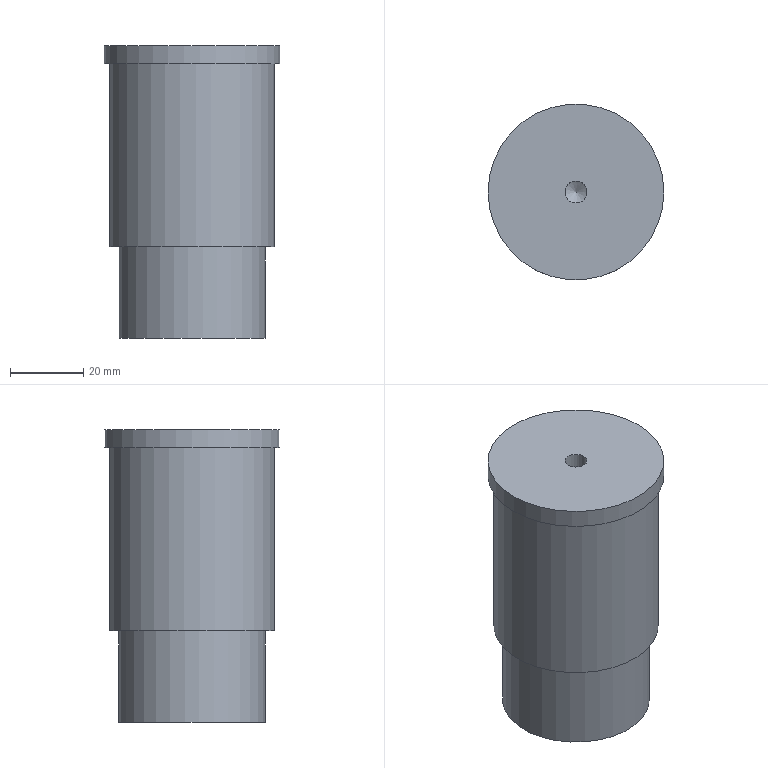Part | NX | features solid 2 | 1 solid | 9 faces | box 48 x 48 x 80 mm | volume 119601 mm3 | cylinder 4 | plane 4 | cone 1 | commonest cylinder face diameters 6 x1 40 x1 45 x1 48 x1
STEP:
#1=CARTESIAN_POINT('',(117.5,45.006,-8.));
#2=VERTEX_POINT('',#1);
#3=CARTESIAN_POINT('',(95.,45.006,-8.));
#4=DIRECTION('',(0.,0.,1.));
#5=DIRECTION('',(1.,0.,0.));
#6=AXIS2_PLACEMENT_3D('',#3,#4,#5);
#7=CIRCLE('',#6,22.5);
#8=EDGE_CURVE('',#2,#2,#7,.T.);
#9=ORIENTED_EDGE('',*,*,#8,.T.);
#10=EDGE_LOOP('',(#9));
#11=FACE_BOUND('',#10,.T.);
#12=CARTESIAN_POINT('',(117.5,45.006,42.));
#13=VERTEX_POINT('',#12);
#14=CARTESIAN_POINT('',(95.,45.006,42.));
#15=DIRECTION('',(0.,0.,1.));
#16=DIRECTION('',(1.,0.,0.));
#17=AXIS2_PLACEMENT_3D('',#14,#15,#16);
#18=CIRCLE('',#17,22.5);
#19=EDGE_CURVE('',#13,#13,#18,.T.);
#20=ORIENTED_EDGE('',*,*,#19,.F.);
#21=EDGE_LOOP('',(#20));
#22=FACE_BOUND('',#21,.T.);
#23=CARTESIAN_POINT('',(95.,45.006,47.));
#24=DIRECTION('',(0.,0.,-1.));
#25=DIRECTION('',(-1.,0.,0.));
#26=AXIS2_PLACEMENT_3D('',#23,#24,#25);
#27=CYLINDRICAL_SURFACE('',#26,22.5);
#28=ADVANCED_FACE('',(#11,#22),#27,.T.);
#29=CARTESIAN_POINT('',(115.,45.006,-8.));
#30=VERTEX_POINT('',#29);
#31=CARTESIAN_POINT('',(95.,45.006,-8.));
#32=DIRECTION('',(0.,0.,1.));
#33=DIRECTION('',(1.,0.,0.));
#34=AXIS2_PLACEMENT_3D('',#31,#32,#33);
#35=CIRCLE('',#34,20.);
#36=EDGE_CURVE('',#30,#30,#35,.T.);
#37=ORIENTED_EDGE('',*,*,#36,.T.);
#38=EDGE_LOOP('',(#37));
#39=FACE_BOUND('',#38,.T.);
#40=ORIENTED_EDGE('',*,*,#8,.F.);
#41=EDGE_LOOP('',(#40));
#42=FACE_BOUND('',#41,.T.);
#43=CARTESIAN_POINT('',(95.,45.006,-8.));
#44=DIRECTION('',(0.,0.,1.));
#45=DIRECTION('',(1.,0.,0.));
#46=AXIS2_PLACEMENT_3D('',#43,#44,#45);
#47=PLANE('',#46);
#48=ADVANCED_FACE('',(#39,#42),#47,.F.);
#49=CARTESIAN_POINT('',(119.,45.006,42.));
#50=VERTEX_POINT('',#49);
#51=CARTESIAN_POINT('',(95.,45.006,42.));
#52=DIRECTION('',(0.,0.,1.));
#53=DIRECTION('',(1.,0.,0.));
#54=AXIS2_PLACEMENT_3D('',#51,#52,#53);
#55=CIRCLE('',#54,24.);
#56=EDGE_CURVE('',#50,#50,#55,.T.);
#57=ORIENTED_EDGE('',*,*,#56,.F.);
#58=EDGE_LOOP('',(#57));
#59=FACE_BOUND('',#58,.T.);
#60=ORIENTED_EDGE('',*,*,#19,.T.);
#61=EDGE_LOOP('',(#60));
#62=FACE_BOUND('',#61,.T.);
#63=CARTESIAN_POINT('',(95.,45.006,42.));
#64=DIRECTION('',(0.,0.,1.));
#65=DIRECTION('',(1.,0.,0.));
#66=AXIS2_PLACEMENT_3D('',#63,#64,#65);
#67=PLANE('',#66);
#68=ADVANCED_FACE('',(#59,#62),#67,.F.);
#69=ORIENTED_EDGE('',*,*,#56,.T.);
#70=EDGE_LOOP('',(#69));
#71=FACE_BOUND('',#70,.T.);
#72=CARTESIAN_POINT('',(119.,45.006,47.));
#73=VERTEX_POINT('',#72);
#74=CARTESIAN_POINT('',(95.,45.006,47.));
#75=DIRECTION('',(0.,0.,1.));
#76=DIRECTION('',(1.,0.,0.));
#77=AXIS2_PLACEMENT_3D('',#74,#75,#76);
#78=CIRCLE('',#77,24.);
#79=EDGE_CURVE('',#73,#73,#78,.T.);
#80=ORIENTED_EDGE('',*,*,#79,.F.);
#81=EDGE_LOOP('',(#80));
#82=FACE_BOUND('',#81,.T.);
#83=CARTESIAN_POINT('',(95.,45.006,42.));
#84=DIRECTION('',(0.,0.,1.));
#85=DIRECTION('',(1.,0.,0.));
#86=AXIS2_PLACEMENT_3D('',#83,#84,#85);
#87=CYLINDRICAL_SURFACE('',#86,24.);
#88=ADVANCED_FACE('',(#71,#82),#87,.T.);
#89=CARTESIAN_POINT('',(92.,45.006,47.));
#90=VERTEX_POINT('',#89);
#91=CARTESIAN_POINT('',(95.,45.006,47.));
#92=DIRECTION('',(0.,0.,-1.));
#93=DIRECTION('',(-1.,0.,0.));
#94=AXIS2_PLACEMENT_3D('',#91,#92,#93);
#95=CIRCLE('',#94,3.);
#96=EDGE_CURVE('',#90,#90,#95,.T.);
#97=ORIENTED_EDGE('',*,*,#96,.T.);
#98=EDGE_LOOP('',(#97));
#99=FACE_BOUND('',#98,.T.);
#100=ORIENTED_EDGE('',*,*,#79,.T.);
#101=EDGE_LOOP('',(#100));
#102=FACE_BOUND('',#101,.T.);
#103=CARTESIAN_POINT('',(95.,45.006,47.));
#104=DIRECTION('',(0.,0.,1.));
#105=DIRECTION('',(1.,0.,0.));
#106=AXIS2_PLACEMENT_3D('',#103,#104,#105);
#107=PLANE('',#106);
#108=ADVANCED_FACE('',(#99,#102),#107,.T.);
#109=CARTESIAN_POINT('',(115.,45.006,-33.));
#110=VERTEX_POINT('',#109);
#111=CARTESIAN_POINT('',(95.,45.006,-33.));
#112=DIRECTION('',(0.,0.,1.));
#113=DIRECTION('',(1.,0.,0.));
#114=AXIS2_PLACEMENT_3D('',#111,#112,#113);
#115=CIRCLE('',#114,20.);
#116=EDGE_CURVE('',#110,#110,#115,.T.);
#117=ORIENTED_EDGE('',*,*,#116,.T.);
#118=EDGE_LOOP('',(#117));
#119=FACE_BOUND('',#118,.T.);
#120=ORIENTED_EDGE('',*,*,#36,.F.);
#121=EDGE_LOOP('',(#120));
#122=FACE_BOUND('',#121,.T.);
#123=CARTESIAN_POINT('',(95.,45.006,-33.));
#124=DIRECTION('',(0.,0.,1.));
#125=DIRECTION('',(1.,0.,0.));
#126=AXIS2_PLACEMENT_3D('',#123,#124,#125);
#127=CYLINDRICAL_SURFACE('',#126,20.);
#128=ADVANCED_FACE('',(#119,#122),#127,.T.);
#129=ORIENTED_EDGE('',*,*,#116,.F.);
#130=EDGE_LOOP('',(#129));
#131=FACE_BOUND('',#130,.T.);
#132=CARTESIAN_POINT('',(95.,45.006,-33.));
#133=DIRECTION('',(0.,0.,1.));
#134=DIRECTION('',(1.,0.,0.));
#135=AXIS2_PLACEMENT_3D('',#132,#133,#134);
#136=PLANE('',#135);
#137=ADVANCED_FACE('',(#131),#136,.F.);
#138=CARTESIAN_POINT('',(92.,45.006,34.));
#139=VERTEX_POINT('',#138);
#140=CARTESIAN_POINT('',(95.,45.006,34.));
#141=DIRECTION('',(0.,0.,-1.));
#142=DIRECTION('',(-1.,0.,0.));
#143=AXIS2_PLACEMENT_3D('',#140,#141,#142);
#144=CIRCLE('',#143,3.);
#145=EDGE_CURVE('',#139,#139,#144,.T.);
#146=ORIENTED_EDGE('',*,*,#145,.F.);
#147=EDGE_LOOP('',(#146));
#148=FACE_BOUND('',#147,.T.);
#149=CARTESIAN_POINT('',(95.,45.006,32.268));
#150=VERTEX_POINT('',#149);
#151=VERTEX_LOOP('',#150);
#152=FACE_BOUND('',#151,.T.);
#153=CARTESIAN_POINT('',(95.,45.006,34.));
#154=DIRECTION('',(0.,0.,1.));
#155=DIRECTION('',(1.,0.,0.));
#156=AXIS2_PLACEMENT_3D('',#153,#154,#155);
#157=CONICAL_SURFACE('',#156,3.,1.047);
#158=ADVANCED_FACE('',(#148,#152),#157,.F.);
#159=ORIENTED_EDGE('',*,*,#145,.T.);
#160=EDGE_LOOP('',(#159));
#161=FACE_BOUND('',#160,.T.);
#162=ORIENTED_EDGE('',*,*,#96,.F.);
#163=EDGE_LOOP('',(#162));
#164=FACE_BOUND('',#163,.T.);
#165=CARTESIAN_POINT('',(95.,45.006,47.));
#166=DIRECTION('',(0.,0.,-1.));
#167=DIRECTION('',(-1.,0.,0.));
#168=AXIS2_PLACEMENT_3D('',#165,#166,#167);
#169=CYLINDRICAL_SURFACE('',#168,3.);
#170=ADVANCED_FACE('',(#161,#164),#169,.F.);
#171=CLOSED_SHELL('',(#28,#48,#68,#88,#108,#128,#137,#158,#170));
#172=MANIFOLD_SOLID_BREP('',#171);
#173=(LENGTH_UNIT()NAMED_UNIT(*)SI_UNIT(.MILLI.,.METRE.));
#174=UNCERTAINTY_MEASURE_WITH_UNIT(LENGTH_MEASURE(0.00001),#173,'','');
#175=(NAMED_UNIT(*)PLANE_ANGLE_UNIT()SI_UNIT($,.RADIAN.));
#176=(NAMED_UNIT(*)SI_UNIT($,.STERADIAN.)SOLID_ANGLE_UNIT());
#177=(GEOMETRIC_REPRESENTATION_CONTEXT(3)GLOBAL_UNCERTAINTY_ASSIGNED_CONTEXT((#174))GLOBAL_UNIT_ASSIGNED_CONTEXT((#173,#175,#176))REPRESENTATION_CONTEXT('',''));
#178=ADVANCED_BREP_SHAPE_REPRESENTATION('',(#172),#177);